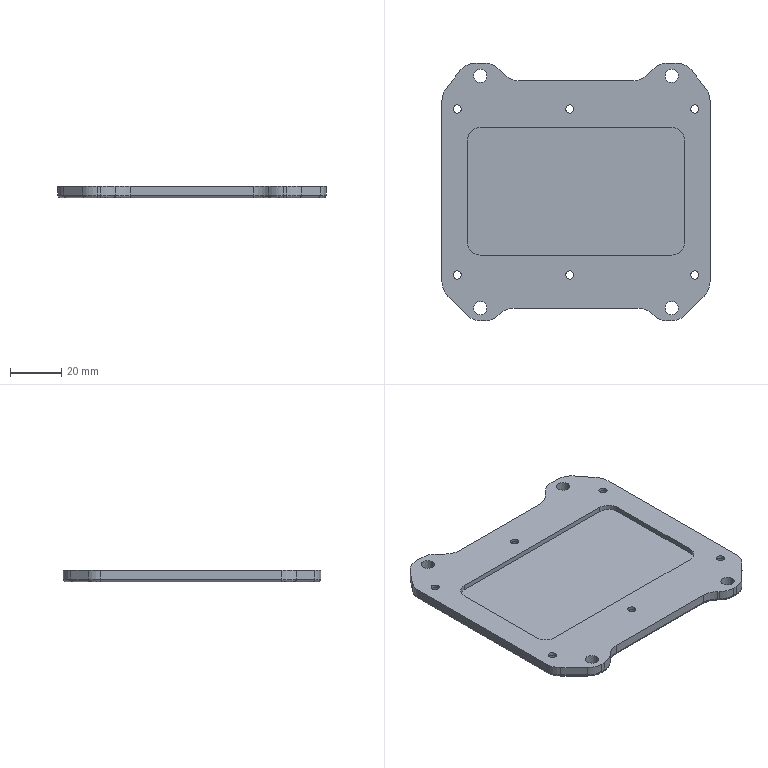Part | 1 solid | 101 faces | box 105 x 101 x 4.5 mm | volume 33851 mm3 | cylinder 56 | plane 29 | torus 16 | commonest cylinder face diameters 2 x16 16 x16 5.2 x8 3.2 x6 5.7 x6 10 x4